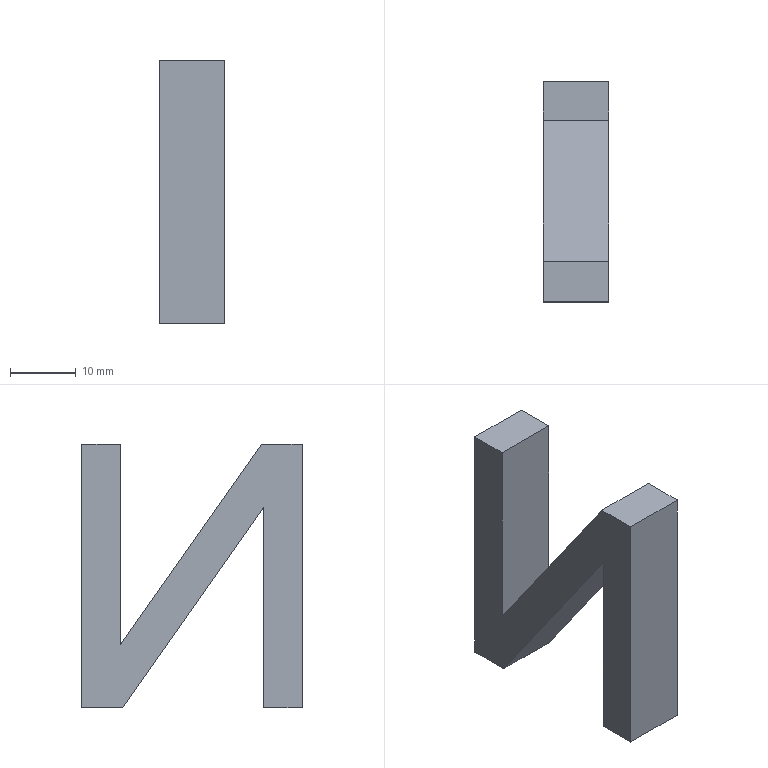Part | NX | features solid 2 | 1 solid | 12 faces | box 10 x 33.468 x 40 mm | volume 6870 mm3 | plane 12
STEP:
#1=CARTESIAN_POINT('',(2250.,-476.141,-590.));
#2=VERTEX_POINT('',#1);
#3=CARTESIAN_POINT('',(2250.,-482.,-590.));
#4=VERTEX_POINT('',#3);
#5=CARTESIAN_POINT('',(2250.,-476.141,-590.));
#6=CARTESIAN_POINT('',(2250.,-478.094,-590.));
#7=CARTESIAN_POINT('',(2250.,-480.047,-590.));
#8=CARTESIAN_POINT('',(2250.,-482.,-590.));
#9=B_SPLINE_CURVE_WITH_KNOTS('',3,(#5,#6,#7,#8),.UNSPECIFIED.,.F.,.F.,(4,4),(0.,0.02446),.PIECEWISE_BEZIER_KNOTS.);
#10=EDGE_CURVE('',#2,#4,#9,.T.);
#11=ORIENTED_EDGE('',*,*,#10,.F.);
#12=CARTESIAN_POINT('',(2260.,-476.141,-590.));
#13=VERTEX_POINT('',#12);
#14=CARTESIAN_POINT('',(2260.,-476.141,-590.));
#15=DIRECTION('',(-1.,0.,0.));
#16=VECTOR('',#15,1000.);
#17=LINE('',#14,#16);
#18=EDGE_CURVE('',#13,#2,#17,.T.);
#19=ORIENTED_EDGE('',*,*,#18,.F.);
#20=CARTESIAN_POINT('',(2260.,-482.,-590.));
#21=VERTEX_POINT('',#20);
#22=CARTESIAN_POINT('',(2260.,-476.141,-590.));
#23=CARTESIAN_POINT('',(2260.,-478.094,-590.));
#24=CARTESIAN_POINT('',(2260.,-480.047,-590.));
#25=CARTESIAN_POINT('',(2260.,-482.,-590.));
#26=B_SPLINE_CURVE_WITH_KNOTS('',3,(#22,#23,#24,#25),.UNSPECIFIED.,.F.,.F.,(4,4),(0.,0.02446),.PIECEWISE_BEZIER_KNOTS.);
#27=EDGE_CURVE('',#13,#21,#26,.T.);
#28=ORIENTED_EDGE('',*,*,#27,.T.);
#29=CARTESIAN_POINT('',(2260.,-482.,-590.));
#30=DIRECTION('',(-1.,0.,0.));
#31=VECTOR('',#30,1000.);
#32=LINE('',#29,#31);
#33=EDGE_CURVE('',#21,#4,#32,.T.);
#34=ORIENTED_EDGE('',*,*,#33,.T.);
#35=EDGE_LOOP('',(#11,#19,#28,#34));
#36=FACE_BOUND('',#35,.T.);
#37=CARTESIAN_POINT('',(2260.,-476.141,-590.));
#38=DIRECTION('',(0.,0.,-1.));
#39=DIRECTION('',(-1.,0.,0.));
#40=AXIS2_PLACEMENT_3D('',#37,#38,#39);
#41=PLANE('',#40);
#42=ADVANCED_FACE('',(#36),#41,.T.);
#43=CARTESIAN_POINT('',(2250.,-482.,-550.));
#44=VERTEX_POINT('',#43);
#45=CARTESIAN_POINT('',(2250.,-482.,-590.));
#46=CARTESIAN_POINT('',(2250.,-482.,-576.667));
#47=CARTESIAN_POINT('',(2250.,-482.,-563.333));
#48=CARTESIAN_POINT('',(2250.,-482.,-550.));
#49=B_SPLINE_CURVE_WITH_KNOTS('',3,(#45,#46,#47,#48),.UNSPECIFIED.,.F.,.F.,(4,4),(0.02446,0.1915),.PIECEWISE_BEZIER_KNOTS.);
#50=EDGE_CURVE('',#4,#44,#49,.T.);
#51=ORIENTED_EDGE('',*,*,#50,.F.);
#52=ORIENTED_EDGE('',*,*,#33,.F.);
#53=CARTESIAN_POINT('',(2260.,-482.,-550.));
#54=VERTEX_POINT('',#53);
#55=CARTESIAN_POINT('',(2260.,-482.,-590.));
#56=CARTESIAN_POINT('',(2260.,-482.,-576.667));
#57=CARTESIAN_POINT('',(2260.,-482.,-563.333));
#58=CARTESIAN_POINT('',(2260.,-482.,-550.));
#59=B_SPLINE_CURVE_WITH_KNOTS('',3,(#55,#56,#57,#58),.UNSPECIFIED.,.F.,.F.,(4,4),(0.02446,0.1915),.PIECEWISE_BEZIER_KNOTS.);
#60=EDGE_CURVE('',#21,#54,#59,.T.);
#61=ORIENTED_EDGE('',*,*,#60,.T.);
#62=CARTESIAN_POINT('',(2260.,-482.,-550.));
#63=DIRECTION('',(-1.,0.,0.));
#64=VECTOR('',#63,1000.);
#65=LINE('',#62,#64);
#66=EDGE_CURVE('',#54,#44,#65,.T.);
#67=ORIENTED_EDGE('',*,*,#66,.T.);
#68=EDGE_LOOP('',(#51,#52,#61,#67));
#69=FACE_BOUND('',#68,.T.);
#70=CARTESIAN_POINT('',(2260.,-482.,-590.));
#71=DIRECTION('',(0.,-1.,0.));
#72=DIRECTION('',(1.,0.,0.));
#73=AXIS2_PLACEMENT_3D('',#70,#71,#72);
#74=PLANE('',#73);
#75=ADVANCED_FACE('',(#69),#74,.T.);
#76=CARTESIAN_POINT('',(2250.,-475.805,-550.));
#77=VERTEX_POINT('',#76);
#78=CARTESIAN_POINT('',(2250.,-482.,-550.));
#79=CARTESIAN_POINT('',(2250.,-479.935,-550.));
#80=CARTESIAN_POINT('',(2250.,-477.87,-550.));
#81=CARTESIAN_POINT('',(2250.,-475.805,-550.));
#82=B_SPLINE_CURVE_WITH_KNOTS('',3,(#78,#79,#80,#81),.UNSPECIFIED.,.F.,.F.,(4,4),(0.1915,0.2174),.PIECEWISE_BEZIER_KNOTS.);
#83=EDGE_CURVE('',#44,#77,#82,.T.);
#84=ORIENTED_EDGE('',*,*,#83,.F.);
#85=ORIENTED_EDGE('',*,*,#66,.F.);
#86=CARTESIAN_POINT('',(2260.,-475.805,-550.));
#87=VERTEX_POINT('',#86);
#88=CARTESIAN_POINT('',(2260.,-482.,-550.));
#89=CARTESIAN_POINT('',(2260.,-479.935,-550.));
#90=CARTESIAN_POINT('',(2260.,-477.87,-550.));
#91=CARTESIAN_POINT('',(2260.,-475.805,-550.));
#92=B_SPLINE_CURVE_WITH_KNOTS('',3,(#88,#89,#90,#91),.UNSPECIFIED.,.F.,.F.,(4,4),(0.1915,0.2174),.PIECEWISE_BEZIER_KNOTS.);
#93=EDGE_CURVE('',#54,#87,#92,.T.);
#94=ORIENTED_EDGE('',*,*,#93,.T.);
#95=CARTESIAN_POINT('',(2260.,-475.805,-550.));
#96=DIRECTION('',(-1.,0.,0.));
#97=VECTOR('',#96,1000.);
#98=LINE('',#95,#97);
#99=EDGE_CURVE('',#87,#77,#98,.T.);
#100=ORIENTED_EDGE('',*,*,#99,.T.);
#101=EDGE_LOOP('',(#84,#85,#94,#100));
#102=FACE_BOUND('',#101,.T.);
#103=CARTESIAN_POINT('',(2260.,-482.,-550.));
#104=DIRECTION('',(0.,0.,1.));
#105=DIRECTION('',(1.,0.,0.));
#106=AXIS2_PLACEMENT_3D('',#103,#104,#105);
#107=PLANE('',#106);
#108=ADVANCED_FACE('',(#102),#107,.T.);
#109=CARTESIAN_POINT('',(2250.,-454.39,-580.47));
#110=VERTEX_POINT('',#109);
#111=CARTESIAN_POINT('',(2250.,-475.805,-550.));
#112=CARTESIAN_POINT('',(2250.,-468.667,-560.157));
#113=CARTESIAN_POINT('',(2250.,-461.528,-570.314));
#114=CARTESIAN_POINT('',(2250.,-454.39,-580.47));
#115=B_SPLINE_CURVE_WITH_KNOTS('',3,(#111,#112,#113,#114),.UNSPECIFIED.,.F.,.F.,(4,4),(0.2174,0.3729),.PIECEWISE_BEZIER_KNOTS.);
#116=EDGE_CURVE('',#77,#110,#115,.T.);
#117=ORIENTED_EDGE('',*,*,#116,.F.);
#118=ORIENTED_EDGE('',*,*,#99,.F.);
#119=CARTESIAN_POINT('',(2260.,-454.39,-580.47));
#120=VERTEX_POINT('',#119);
#121=CARTESIAN_POINT('',(2260.,-475.805,-550.));
#122=CARTESIAN_POINT('',(2260.,-468.667,-560.157));
#123=CARTESIAN_POINT('',(2260.,-461.528,-570.314));
#124=CARTESIAN_POINT('',(2260.,-454.39,-580.47));
#125=B_SPLINE_CURVE_WITH_KNOTS('',3,(#121,#122,#123,#124),.UNSPECIFIED.,.F.,.F.,(4,4),(0.2174,0.3729),.PIECEWISE_BEZIER_KNOTS.);
#126=EDGE_CURVE('',#87,#120,#125,.T.);
#127=ORIENTED_EDGE('',*,*,#126,.T.);
#128=CARTESIAN_POINT('',(2260.,-454.39,-580.47));
#129=DIRECTION('',(-1.,0.,0.));
#130=VECTOR('',#129,1000.);
#131=LINE('',#128,#130);
#132=EDGE_CURVE('',#120,#110,#131,.T.);
#133=ORIENTED_EDGE('',*,*,#132,.T.);
#134=EDGE_LOOP('',(#117,#118,#127,#133));
#135=FACE_BOUND('',#134,.T.);
#136=CARTESIAN_POINT('',(2260.,-475.805,-550.));
#137=DIRECTION('',(0.,0.8181,0.575));
#138=DIRECTION('',(0.,-0.575,0.8181));
#139=AXIS2_PLACEMENT_3D('',#136,#137,#138);
#140=PLANE('',#139);
#141=ADVANCED_FACE('',(#135),#140,.T.);
#142=CARTESIAN_POINT('',(2250.,-454.39,-550.));
#143=VERTEX_POINT('',#142);
#144=CARTESIAN_POINT('',(2250.,-454.39,-580.47));
#145=CARTESIAN_POINT('',(2250.,-454.39,-570.314));
#146=CARTESIAN_POINT('',(2250.,-454.39,-560.157));
#147=CARTESIAN_POINT('',(2250.,-454.39,-550.));
#148=B_SPLINE_CURVE_WITH_KNOTS('',3,(#144,#145,#146,#147),.UNSPECIFIED.,.F.,.F.,(4,4),(0.3729,0.5001),.PIECEWISE_BEZIER_KNOTS.);
#149=EDGE_CURVE('',#110,#143,#148,.T.);
#150=ORIENTED_EDGE('',*,*,#149,.F.);
#151=ORIENTED_EDGE('',*,*,#132,.F.);
#152=CARTESIAN_POINT('',(2260.,-454.39,-550.));
#153=VERTEX_POINT('',#152);
#154=CARTESIAN_POINT('',(2260.,-454.39,-580.47));
#155=CARTESIAN_POINT('',(2260.,-454.39,-570.314));
#156=CARTESIAN_POINT('',(2260.,-454.39,-560.157));
#157=CARTESIAN_POINT('',(2260.,-454.39,-550.));
#158=B_SPLINE_CURVE_WITH_KNOTS('',3,(#154,#155,#156,#157),.UNSPECIFIED.,.F.,.F.,(4,4),(0.3729,0.5001),.PIECEWISE_BEZIER_KNOTS.);
#159=EDGE_CURVE('',#120,#153,#158,.T.);
#160=ORIENTED_EDGE('',*,*,#159,.T.);
#161=CARTESIAN_POINT('',(2260.,-454.39,-550.));
#162=DIRECTION('',(-1.,0.,0.));
#163=VECTOR('',#162,1000.);
#164=LINE('',#161,#163);
#165=EDGE_CURVE('',#153,#143,#164,.T.);
#166=ORIENTED_EDGE('',*,*,#165,.T.);
#167=EDGE_LOOP('',(#150,#151,#160,#166));
#168=FACE_BOUND('',#167,.T.);
#169=CARTESIAN_POINT('',(2260.,-454.39,-580.47));
#170=DIRECTION('',(0.,-1.,0.));
#171=DIRECTION('',(1.,0.,0.));
#172=AXIS2_PLACEMENT_3D('',#169,#170,#171);
#173=PLANE('',#172);
#174=ADVANCED_FACE('',(#168),#173,.T.);
#175=CARTESIAN_POINT('',(2250.,-448.532,-550.));
#176=VERTEX_POINT('',#175);
#177=CARTESIAN_POINT('',(2250.,-454.39,-550.));
#178=CARTESIAN_POINT('',(2250.,-452.437,-550.));
#179=CARTESIAN_POINT('',(2250.,-450.484,-550.));
#180=CARTESIAN_POINT('',(2250.,-448.532,-550.));
#181=B_SPLINE_CURVE_WITH_KNOTS('',3,(#177,#178,#179,#180),.UNSPECIFIED.,.F.,.F.,(4,4),(0.5001,0.5246),.PIECEWISE_BEZIER_KNOTS.);
#182=EDGE_CURVE('',#143,#176,#181,.T.);
#183=ORIENTED_EDGE('',*,*,#182,.F.);
#184=ORIENTED_EDGE('',*,*,#165,.F.);
#185=CARTESIAN_POINT('',(2260.,-448.532,-550.));
#186=VERTEX_POINT('',#185);
#187=CARTESIAN_POINT('',(2260.,-454.39,-550.));
#188=CARTESIAN_POINT('',(2260.,-452.437,-550.));
#189=CARTESIAN_POINT('',(2260.,-450.484,-550.));
#190=CARTESIAN_POINT('',(2260.,-448.532,-550.));
#191=B_SPLINE_CURVE_WITH_KNOTS('',3,(#187,#188,#189,#190),.UNSPECIFIED.,.F.,.F.,(4,4),(0.5001,0.5246),.PIECEWISE_BEZIER_KNOTS.);
#192=EDGE_CURVE('',#153,#186,#191,.T.);
#193=ORIENTED_EDGE('',*,*,#192,.T.);
#194=CARTESIAN_POINT('',(2260.,-448.532,-550.));
#195=DIRECTION('',(-1.,0.,0.));
#196=VECTOR('',#195,1000.);
#197=LINE('',#194,#196);
#198=EDGE_CURVE('',#186,#176,#197,.T.);
#199=ORIENTED_EDGE('',*,*,#198,.T.);
#200=EDGE_LOOP('',(#183,#184,#193,#199));
#201=FACE_BOUND('',#200,.T.);
#202=CARTESIAN_POINT('',(2260.,-454.39,-550.));
#203=DIRECTION('',(0.,0.,1.));
#204=DIRECTION('',(1.,0.,0.));
#205=AXIS2_PLACEMENT_3D('',#202,#203,#204);
#206=PLANE('',#205);
#207=ADVANCED_FACE('',(#201),#206,.T.);
#208=CARTESIAN_POINT('',(2250.,-448.532,-590.));
#209=VERTEX_POINT('',#208);
#210=CARTESIAN_POINT('',(2250.,-448.532,-550.));
#211=CARTESIAN_POINT('',(2250.,-448.532,-563.333));
#212=CARTESIAN_POINT('',(2250.,-448.532,-576.667));
#213=CARTESIAN_POINT('',(2250.,-448.532,-590.));
#214=B_SPLINE_CURVE_WITH_KNOTS('',3,(#210,#211,#212,#213),.UNSPECIFIED.,.F.,.F.,(4,4),(0.5246,0.6916),.PIECEWISE_BEZIER_KNOTS.);
#215=EDGE_CURVE('',#176,#209,#214,.T.);
#216=ORIENTED_EDGE('',*,*,#215,.F.);
#217=ORIENTED_EDGE('',*,*,#198,.F.);
#218=CARTESIAN_POINT('',(2260.,-448.532,-590.));
#219=VERTEX_POINT('',#218);
#220=CARTESIAN_POINT('',(2260.,-448.532,-550.));
#221=CARTESIAN_POINT('',(2260.,-448.532,-563.333));
#222=CARTESIAN_POINT('',(2260.,-448.532,-576.667));
#223=CARTESIAN_POINT('',(2260.,-448.532,-590.));
#224=B_SPLINE_CURVE_WITH_KNOTS('',3,(#220,#221,#222,#223),.UNSPECIFIED.,.F.,.F.,(4,4),(0.5246,0.6916),.PIECEWISE_BEZIER_KNOTS.);
#225=EDGE_CURVE('',#186,#219,#224,.T.);
#226=ORIENTED_EDGE('',*,*,#225,.T.);
#227=CARTESIAN_POINT('',(2260.,-448.532,-590.));
#228=DIRECTION('',(-1.,0.,0.));
#229=VECTOR('',#228,1000.);
#230=LINE('',#227,#229);
#231=EDGE_CURVE('',#219,#209,#230,.T.);
#232=ORIENTED_EDGE('',*,*,#231,.T.);
#233=EDGE_LOOP('',(#216,#217,#226,#232));
#234=FACE_BOUND('',#233,.T.);
#235=CARTESIAN_POINT('',(2260.,-448.532,-550.));
#236=DIRECTION('',(0.,1.,0.));
#237=DIRECTION('',(-1.,0.,0.));
#238=AXIS2_PLACEMENT_3D('',#235,#236,#237);
#239=PLANE('',#238);
#240=ADVANCED_FACE('',(#234),#239,.T.);
#241=CARTESIAN_POINT('',(2250.,-454.757,-590.));
#242=VERTEX_POINT('',#241);
#243=CARTESIAN_POINT('',(2250.,-448.532,-590.));
#244=CARTESIAN_POINT('',(2250.,-450.607,-590.));
#245=CARTESIAN_POINT('',(2250.,-452.682,-590.));
#246=CARTESIAN_POINT('',(2250.,-454.757,-590.));
#247=B_SPLINE_CURVE_WITH_KNOTS('',3,(#243,#244,#245,#246),.UNSPECIFIED.,.F.,.F.,(4,4),(0.6916,0.7176),.PIECEWISE_BEZIER_KNOTS.);
#248=EDGE_CURVE('',#209,#242,#247,.T.);
#249=ORIENTED_EDGE('',*,*,#248,.F.);
#250=ORIENTED_EDGE('',*,*,#231,.F.);
#251=CARTESIAN_POINT('',(2260.,-454.757,-590.));
#252=VERTEX_POINT('',#251);
#253=CARTESIAN_POINT('',(2260.,-448.532,-590.));
#254=CARTESIAN_POINT('',(2260.,-450.607,-590.));
#255=CARTESIAN_POINT('',(2260.,-452.682,-590.));
#256=CARTESIAN_POINT('',(2260.,-454.757,-590.));
#257=B_SPLINE_CURVE_WITH_KNOTS('',3,(#253,#254,#255,#256),.UNSPECIFIED.,.F.,.F.,(4,4),(0.6916,0.7176),.PIECEWISE_BEZIER_KNOTS.);
#258=EDGE_CURVE('',#219,#252,#257,.T.);
#259=ORIENTED_EDGE('',*,*,#258,.T.);
#260=CARTESIAN_POINT('',(2260.,-454.757,-590.));
#261=DIRECTION('',(-1.,0.,0.));
#262=VECTOR('',#261,1000.);
#263=LINE('',#260,#262);
#264=EDGE_CURVE('',#252,#242,#263,.T.);
#265=ORIENTED_EDGE('',*,*,#264,.T.);
#266=EDGE_LOOP('',(#249,#250,#259,#265));
#267=FACE_BOUND('',#266,.T.);
#268=CARTESIAN_POINT('',(2260.,-448.532,-590.));
#269=DIRECTION('',(0.,0.,-1.));
#270=DIRECTION('',(-1.,0.,0.));
#271=AXIS2_PLACEMENT_3D('',#268,#269,#270);
#272=PLANE('',#271);
#273=ADVANCED_FACE('',(#267),#272,.T.);
#274=CARTESIAN_POINT('',(2250.,-476.141,-559.56));
#275=VERTEX_POINT('',#274);
#276=CARTESIAN_POINT('',(2250.,-454.757,-590.));
#277=CARTESIAN_POINT('',(2250.,-461.885,-579.853));
#278=CARTESIAN_POINT('',(2250.,-469.013,-569.707));
#279=CARTESIAN_POINT('',(2250.,-476.141,-559.56));
#280=B_SPLINE_CURVE_WITH_KNOTS('',3,(#276,#277,#278,#279),.UNSPECIFIED.,.F.,.F.,(4,4),(0.7176,0.8729),.PIECEWISE_BEZIER_KNOTS.);
#281=EDGE_CURVE('',#242,#275,#280,.T.);
#282=ORIENTED_EDGE('',*,*,#281,.F.);
#283=ORIENTED_EDGE('',*,*,#264,.F.);
#284=CARTESIAN_POINT('',(2260.,-476.141,-559.56));
#285=VERTEX_POINT('',#284);
#286=CARTESIAN_POINT('',(2260.,-454.757,-590.));
#287=CARTESIAN_POINT('',(2260.,-461.885,-579.853));
#288=CARTESIAN_POINT('',(2260.,-469.013,-569.707));
#289=CARTESIAN_POINT('',(2260.,-476.141,-559.56));
#290=B_SPLINE_CURVE_WITH_KNOTS('',3,(#286,#287,#288,#289),.UNSPECIFIED.,.F.,.F.,(4,4),(0.7176,0.8729),.PIECEWISE_BEZIER_KNOTS.);
#291=EDGE_CURVE('',#252,#285,#290,.T.);
#292=ORIENTED_EDGE('',*,*,#291,.T.);
#293=CARTESIAN_POINT('',(2260.,-476.141,-559.56));
#294=DIRECTION('',(-1.,0.,0.));
#295=VECTOR('',#294,1000.);
#296=LINE('',#293,#295);
#297=EDGE_CURVE('',#285,#275,#296,.T.);
#298=ORIENTED_EDGE('',*,*,#297,.T.);
#299=EDGE_LOOP('',(#282,#283,#292,#298));
#300=FACE_BOUND('',#299,.T.);
#301=CARTESIAN_POINT('',(2260.,-454.757,-590.));
#302=DIRECTION('',(0.,-0.8183,-0.5748));
#303=DIRECTION('',(0.,0.5748,-0.8183));
#304=AXIS2_PLACEMENT_3D('',#301,#302,#303);
#305=PLANE('',#304);
#306=ADVANCED_FACE('',(#300),#305,.T.);
#307=CARTESIAN_POINT('',(2250.,-476.141,-559.56));
#308=CARTESIAN_POINT('',(2250.,-476.141,-569.707));
#309=CARTESIAN_POINT('',(2250.,-476.141,-579.853));
#310=CARTESIAN_POINT('',(2250.,-476.141,-590.));
#311=B_SPLINE_CURVE_WITH_KNOTS('',3,(#307,#308,#309,#310),.UNSPECIFIED.,.F.,.F.,(4,4),(0.8729,1.),.PIECEWISE_BEZIER_KNOTS.);
#312=EDGE_CURVE('',#275,#2,#311,.T.);
#313=ORIENTED_EDGE('',*,*,#312,.F.);
#314=ORIENTED_EDGE('',*,*,#297,.F.);
#315=CARTESIAN_POINT('',(2260.,-476.141,-559.56));
#316=CARTESIAN_POINT('',(2260.,-476.141,-569.707));
#317=CARTESIAN_POINT('',(2260.,-476.141,-579.853));
#318=CARTESIAN_POINT('',(2260.,-476.141,-590.));
#319=B_SPLINE_CURVE_WITH_KNOTS('',3,(#315,#316,#317,#318),.UNSPECIFIED.,.F.,.F.,(4,4),(0.8729,1.),.PIECEWISE_BEZIER_KNOTS.);
#320=EDGE_CURVE('',#285,#13,#319,.T.);
#321=ORIENTED_EDGE('',*,*,#320,.T.);
#322=ORIENTED_EDGE('',*,*,#18,.T.);
#323=EDGE_LOOP('',(#313,#314,#321,#322));
#324=FACE_BOUND('',#323,.T.);
#325=CARTESIAN_POINT('',(2260.,-476.141,-559.56));
#326=DIRECTION('',(0.,1.,0.));
#327=DIRECTION('',(-1.,0.,0.));
#328=AXIS2_PLACEMENT_3D('',#325,#326,#327);
#329=PLANE('',#328);
#330=ADVANCED_FACE('',(#324),#329,.T.);
#331=ORIENTED_EDGE('',*,*,#27,.F.);
#332=ORIENTED_EDGE('',*,*,#320,.F.);
#333=ORIENTED_EDGE('',*,*,#291,.F.);
#334=ORIENTED_EDGE('',*,*,#258,.F.);
#335=ORIENTED_EDGE('',*,*,#225,.F.);
#336=ORIENTED_EDGE('',*,*,#192,.F.);
#337=ORIENTED_EDGE('',*,*,#159,.F.);
#338=ORIENTED_EDGE('',*,*,#126,.F.);
#339=ORIENTED_EDGE('',*,*,#93,.F.);
#340=ORIENTED_EDGE('',*,*,#60,.F.);
#341=EDGE_LOOP('',(#331,#332,#333,#334,#335,#336,#337,#338,#339,#340));
#342=FACE_BOUND('',#341,.T.);
#343=CARTESIAN_POINT('',(2260.,-479.071,-590.));
#344=DIRECTION('',(1.,0.,0.));
#345=DIRECTION('',(0.,1.,0.));
#346=AXIS2_PLACEMENT_3D('',#343,#344,#345);
#347=PLANE('',#346);
#348=ADVANCED_FACE('',(#342),#347,.T.);
#349=ORIENTED_EDGE('',*,*,#10,.T.);
#350=ORIENTED_EDGE('',*,*,#50,.T.);
#351=ORIENTED_EDGE('',*,*,#83,.T.);
#352=ORIENTED_EDGE('',*,*,#116,.T.);
#353=ORIENTED_EDGE('',*,*,#149,.T.);
#354=ORIENTED_EDGE('',*,*,#182,.T.);
#355=ORIENTED_EDGE('',*,*,#215,.T.);
#356=ORIENTED_EDGE('',*,*,#248,.T.);
#357=ORIENTED_EDGE('',*,*,#281,.T.);
#358=ORIENTED_EDGE('',*,*,#312,.T.);
#359=EDGE_LOOP('',(#349,#350,#351,#352,#353,#354,#355,#356,#357,#358));
#360=FACE_BOUND('',#359,.T.);
#361=CARTESIAN_POINT('',(2250.,-479.071,-590.));
#362=DIRECTION('',(1.,0.,0.));
#363=DIRECTION('',(0.,1.,0.));
#364=AXIS2_PLACEMENT_3D('',#361,#362,#363);
#365=PLANE('',#364);
#366=ADVANCED_FACE('',(#360),#365,.F.);
#367=CLOSED_SHELL('',(#42,#75,#108,#141,#174,#207,#240,#273,#306,#330,#348,#366));
#368=MANIFOLD_SOLID_BREP('',#367);
#369=(LENGTH_UNIT()NAMED_UNIT(*)SI_UNIT(.MILLI.,.METRE.));
#370=UNCERTAINTY_MEASURE_WITH_UNIT(LENGTH_MEASURE(0.00001),#369,'','');
#371=(NAMED_UNIT(*)PLANE_ANGLE_UNIT()SI_UNIT($,.RADIAN.));
#372=(NAMED_UNIT(*)SI_UNIT($,.STERADIAN.)SOLID_ANGLE_UNIT());
#373=(GEOMETRIC_REPRESENTATION_CONTEXT(3)GLOBAL_UNCERTAINTY_ASSIGNED_CONTEXT((#370))GLOBAL_UNIT_ASSIGNED_CONTEXT((#369,#371,#372))REPRESENTATION_CONTEXT('',''));
#374=ADVANCED_BREP_SHAPE_REPRESENTATION('',(#368),#373);